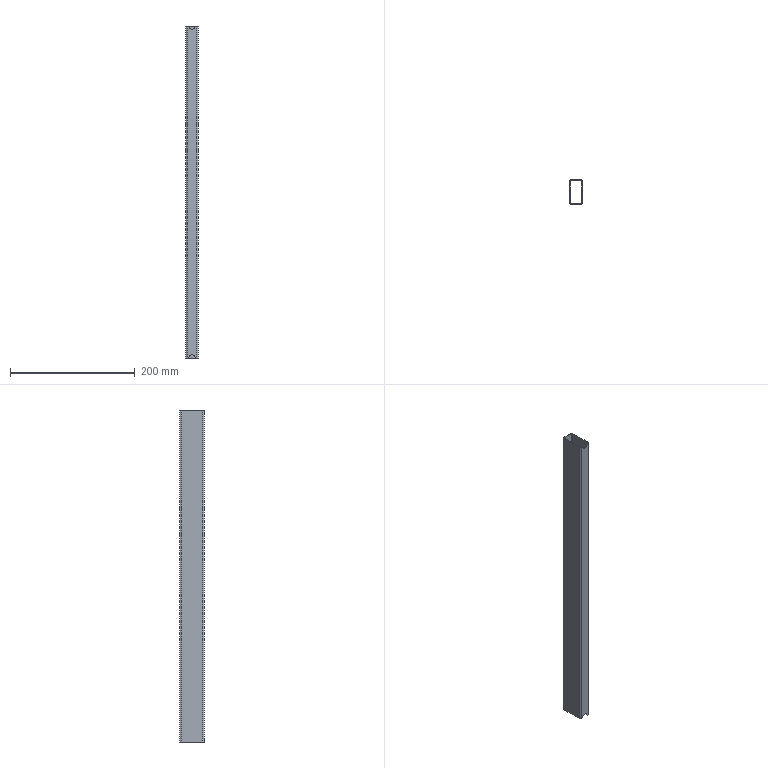Part | STEP file | PN_0007 default | 1 solid | 20 faces | box 20 x 40 x 532 mm | volume 88457 mm3 | plane 10 | cylinder 10 | commonest cylinder face diameters 2 x4 5 x4 10 x2